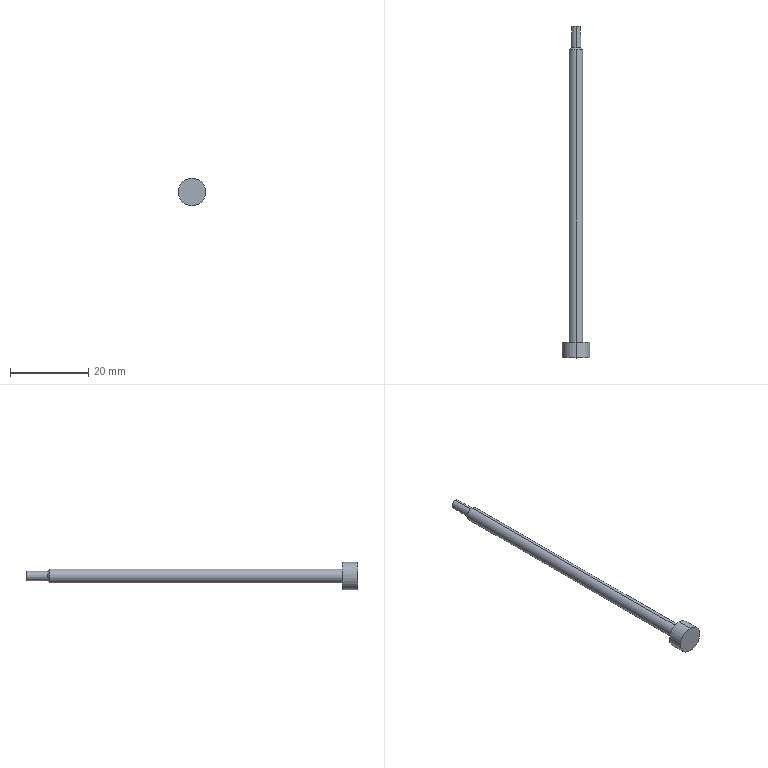Part | STEP file | 1 solid | 11 faces | box 7 x 84.723 x 7 mm | volume 901.172 mm3 | cylinder 4 | cone 4 | plane 3 | commonest cylinder face diameters 3.5 x2 7 x2
STEP:
#1=CARTESIAN_POINT('',(0.,0.,0.));
#2=DIRECTION('',(0.,0.,1.));
#3=DIRECTION('',(1.,0.,0.));
#4=AXIS2_PLACEMENT_3D('',#1,#2,#3);
#5=CARTESIAN_POINT('',(-48.742,-40.,118.07));
#6=VERTEX_POINT('',#5);
#7=CARTESIAN_POINT('',(-48.742,-40.,111.07));
#8=VERTEX_POINT('',#7);
#9=CARTESIAN_POINT('',(-48.742,-40.,114.57));
#10=DIRECTION('',(0.,1.,0.));
#11=DIRECTION('',(0.,0.,-1.));
#12=AXIS2_PLACEMENT_3D('',#9,#10,#11);
#13=CIRCLE('',#12,3.5);
#14=CARTESIAN_POINT('',(-48.742,-50.,114.57));
#15=DIRECTION('',(0.,1.,0.));
#16=DIRECTION('',(0.,0.,1.));
#17=AXIS2_PLACEMENT_3D('',#14,#15,#16);
#18=CYLINDRICAL_SURFACE('',#17,3.5);
#19=CARTESIAN_POINT('',(-3.142,10.));
#20=DIRECTION('',(1.,0.));
#21=VECTOR('',#20,1.);
#22=LINE('',#19,#21);
#23=(GEOMETRIC_REPRESENTATION_CONTEXT(2)PARAMETRIC_REPRESENTATION_CONTEXT()REPRESENTATION_CONTEXT('',''));
#24=DEFINITIONAL_REPRESENTATION('',(#22),#23);
#25=PCURVE('',#18,#24);
#26=CARTESIAN_POINT('',(-72.862,-40.,23.556));
#27=DIRECTION('',(0.,-1.,0.));
#28=DIRECTION('',(0.,0.,-1.));
#29=AXIS2_PLACEMENT_3D('',#26,#27,#28);
#30=PLANE('',#29);
#31=CARTESIAN_POINT('',(-87.514,24.12));
#32=CARTESIAN_POINT('',(-87.514,18.058));
#33=CARTESIAN_POINT('',(-92.764,21.089));
#34=CARTESIAN_POINT('',(-98.014,24.12));
#35=CARTESIAN_POINT('',(-92.764,27.151));
#36=CARTESIAN_POINT('',(-87.514,30.182));
#37=CARTESIAN_POINT('',(-87.514,24.12));
#38=(BOUNDED_CURVE()B_SPLINE_CURVE(2,(#31,#32,#33,#34,#35,#36,#37),.UNSPECIFIED.,.T.,.F.)B_SPLINE_CURVE_WITH_KNOTS((1,2,2,2,2,1),(-2.094,0.,2.094,4.189,6.283,8.378),.UNSPECIFIED.)CURVE()GEOMETRIC_REPRESENTATION_ITEM()RATIONAL_B_SPLINE_CURVE((1.,0.5,1.,0.5,1.,0.5,1.))REPRESENTATION_ITEM(''));
#39=(GEOMETRIC_REPRESENTATION_CONTEXT(2)PARAMETRIC_REPRESENTATION_CONTEXT()REPRESENTATION_CONTEXT('',''));
#40=DEFINITIONAL_REPRESENTATION('',(#38),#39);
#41=PCURVE('',#30,#40);
#42=SURFACE_CURVE('',#13,(#25,#41),.PCURVE_S1.);
#43=EDGE_CURVE('',#6,#8,#42,.T.);
#44=ORIENTED_EDGE('',*,*,#43,.T.);
#45=CARTESIAN_POINT('',(-48.742,-36.,111.07));
#46=VERTEX_POINT('',#45);
#47=CARTESIAN_POINT('',(-48.742,-50.,111.07));
#48=DIRECTION('',(0.,1.,0.));
#49=VECTOR('',#48,1.);
#50=LINE('',#47,#49);
#51=CARTESIAN_POINT('',(3.142,0.));
#52=DIRECTION('',(0.,1.));
#53=VECTOR('',#52,1.);
#54=LINE('',#51,#53);
#55=(GEOMETRIC_REPRESENTATION_CONTEXT(2)PARAMETRIC_REPRESENTATION_CONTEXT()REPRESENTATION_CONTEXT('',''));
#56=DEFINITIONAL_REPRESENTATION('',(#54),#55);
#57=PCURVE('',#18,#56);
#58=CARTESIAN_POINT('',(-48.742,-50.,114.57));
#59=DIRECTION('',(0.,1.,0.));
#60=DIRECTION('',(0.,0.,1.));
#61=AXIS2_PLACEMENT_3D('',#58,#59,#60);
#62=CYLINDRICAL_SURFACE('',#61,3.5);
#63=CARTESIAN_POINT('',(3.142,0.));
#64=DIRECTION('',(0.,1.));
#65=VECTOR('',#64,1.);
#66=LINE('',#63,#65);
#67=(GEOMETRIC_REPRESENTATION_CONTEXT(2)PARAMETRIC_REPRESENTATION_CONTEXT()REPRESENTATION_CONTEXT('',''));
#68=DEFINITIONAL_REPRESENTATION('',(#66),#67);
#69=PCURVE('',#62,#68);
#70=SURFACE_CURVE('',#50,(#57,#69),.PCURVE_S1.);
#71=EDGE_CURVE('',#8,#46,#70,.T.);
#72=ORIENTED_EDGE('',*,*,#71,.T.);
#73=CARTESIAN_POINT('',(-48.742,-36.,118.07));
#74=VERTEX_POINT('',#73);
#75=CARTESIAN_POINT('',(-48.742,-36.,114.57));
#76=DIRECTION('',(0.,-1.,0.));
#77=DIRECTION('',(0.,0.,-1.));
#78=AXIS2_PLACEMENT_3D('',#75,#76,#77);
#79=CIRCLE('',#78,3.5);
#80=CARTESIAN_POINT('',(3.142,14.));
#81=DIRECTION('',(-1.,0.));
#82=VECTOR('',#81,1.);
#83=LINE('',#80,#82);
#84=(GEOMETRIC_REPRESENTATION_CONTEXT(2)PARAMETRIC_REPRESENTATION_CONTEXT()REPRESENTATION_CONTEXT('',''));
#85=DEFINITIONAL_REPRESENTATION('',(#83),#84);
#86=PCURVE('',#18,#85);
#87=CARTESIAN_POINT('',(-48.742,-36.,114.57));
#88=DIRECTION('',(0.,1.,0.));
#89=DIRECTION('',(0.,0.,1.));
#90=AXIS2_PLACEMENT_3D('',#87,#88,#89);
#91=PLANE('',#90);
#92=CARTESIAN_POINT('',(-3.5,0.));
#93=CARTESIAN_POINT('',(-3.5,6.062));
#94=CARTESIAN_POINT('',(1.75,3.031));
#95=CARTESIAN_POINT('',(7.,0.));
#96=CARTESIAN_POINT('',(1.75,-3.031));
#97=CARTESIAN_POINT('',(-3.5,-6.062));
#98=CARTESIAN_POINT('',(-3.5,0.));
#99=(BOUNDED_CURVE()B_SPLINE_CURVE(2,(#92,#93,#94,#95,#96,#97,#98),.UNSPECIFIED.,.T.,.F.)B_SPLINE_CURVE_WITH_KNOTS((1,2,2,2,2,1),(-2.094,0.,2.094,4.189,6.283,8.378),.UNSPECIFIED.)CURVE()GEOMETRIC_REPRESENTATION_ITEM()RATIONAL_B_SPLINE_CURVE((1.,0.5,1.,0.5,1.,0.5,1.))REPRESENTATION_ITEM(''));
#100=(GEOMETRIC_REPRESENTATION_CONTEXT(2)PARAMETRIC_REPRESENTATION_CONTEXT()REPRESENTATION_CONTEXT('',''));
#101=DEFINITIONAL_REPRESENTATION('',(#99),#100);
#102=PCURVE('',#91,#101);
#103=SURFACE_CURVE('',#79,(#86,#102),.PCURVE_S1.);
#104=EDGE_CURVE('',#46,#74,#103,.T.);
#105=ORIENTED_EDGE('',*,*,#104,.T.);
#106=CARTESIAN_POINT('',(-48.742,-50.,118.07));
#107=DIRECTION('',(0.,1.,0.));
#108=VECTOR('',#107,1.);
#109=LINE('',#106,#108);
#110=CARTESIAN_POINT('',(0.,0.));
#111=DIRECTION('',(0.,1.));
#112=VECTOR('',#111,1.);
#113=LINE('',#110,#112);
#114=(GEOMETRIC_REPRESENTATION_CONTEXT(2)PARAMETRIC_REPRESENTATION_CONTEXT()REPRESENTATION_CONTEXT('',''));
#115=DEFINITIONAL_REPRESENTATION('',(#113),#114);
#116=PCURVE('',#18,#115);
#117=CARTESIAN_POINT('',(6.283,0.));
#118=DIRECTION('',(0.,1.));
#119=VECTOR('',#118,1.);
#120=LINE('',#117,#119);
#121=(GEOMETRIC_REPRESENTATION_CONTEXT(2)PARAMETRIC_REPRESENTATION_CONTEXT()REPRESENTATION_CONTEXT('',''));
#122=DEFINITIONAL_REPRESENTATION('',(#120),#121);
#123=PCURVE('',#62,#122);
#124=SURFACE_CURVE('',#109,(#116,#123),.PCURVE_S1.);
#125=EDGE_CURVE('',#6,#74,#124,.T.);
#126=ORIENTED_EDGE('',*,*,#125,.F.);
#127=EDGE_LOOP('',(#44,#72,#105,#126));
#128=FACE_BOUND('',#127,.T.);
#129=ADVANCED_FACE('',(#128),#18,.T.);
#130=CARTESIAN_POINT('',(-48.742,38.701,116.32));
#131=VERTEX_POINT('',#130);
#132=CARTESIAN_POINT('',(-48.742,38.701,112.82));
#133=VERTEX_POINT('',#132);
#134=CARTESIAN_POINT('',(-48.742,38.701,114.57));
#135=DIRECTION('',(0.,1.,0.));
#136=DIRECTION('',(0.,0.,-1.));
#137=AXIS2_PLACEMENT_3D('',#134,#135,#136);
#138=CIRCLE('',#137,1.75);
#139=CARTESIAN_POINT('',(-48.742,44.722,114.57));
#140=DIRECTION('',(0.,-1.,0.));
#141=DIRECTION('',(0.,0.,-1.));
#142=AXIS2_PLACEMENT_3D('',#139,#140,#141);
#143=CYLINDRICAL_SURFACE('',#142,1.75);
#144=CARTESIAN_POINT('',(6.283,6.021));
#145=DIRECTION('',(-1.,0.));
#146=VECTOR('',#145,1.);
#147=LINE('',#144,#146);
#148=(GEOMETRIC_REPRESENTATION_CONTEXT(2)PARAMETRIC_REPRESENTATION_CONTEXT()REPRESENTATION_CONTEXT('',''));
#149=DEFINITIONAL_REPRESENTATION('',(#147),#148);
#150=PCURVE('',#143,#149);
#151=CARTESIAN_POINT('',(-48.742,39.204,114.57));
#152=DIRECTION('',(0.,-1.,0.));
#153=DIRECTION('',(0.,0.,-1.));
#154=AXIS2_PLACEMENT_3D('',#151,#152,#153);
#155=CONICAL_SURFACE('',#154,1.247,0.7854);
#156=CARTESIAN_POINT('',(6.283,0.5027));
#157=DIRECTION('',(-1.,0.));
#158=VECTOR('',#157,1.);
#159=LINE('',#156,#158);
#160=(GEOMETRIC_REPRESENTATION_CONTEXT(2)PARAMETRIC_REPRESENTATION_CONTEXT()REPRESENTATION_CONTEXT('',''));
#161=DEFINITIONAL_REPRESENTATION('',(#159),#160);
#162=PCURVE('',#155,#161);
#163=SURFACE_CURVE('',#138,(#150,#162),.PCURVE_S1.);
#164=EDGE_CURVE('',#131,#133,#163,.T.);
#165=ORIENTED_EDGE('',*,*,#164,.F.);
#166=CARTESIAN_POINT('',(-48.742,-36.,116.32));
#167=VERTEX_POINT('',#166);
#168=CARTESIAN_POINT('',(-48.742,44.722,116.32));
#169=DIRECTION('',(0.,-1.,0.));
#170=VECTOR('',#169,1.);
#171=LINE('',#168,#170);
#172=CARTESIAN_POINT('',(3.142,0.));
#173=DIRECTION('',(0.,1.));
#174=VECTOR('',#173,1.);
#175=LINE('',#172,#174);
#176=(GEOMETRIC_REPRESENTATION_CONTEXT(2)PARAMETRIC_REPRESENTATION_CONTEXT()REPRESENTATION_CONTEXT('',''));
#177=DEFINITIONAL_REPRESENTATION('',(#175),#176);
#178=PCURVE('',#143,#177);
#179=CARTESIAN_POINT('',(-48.742,44.722,114.57));
#180=DIRECTION('',(0.,-1.,0.));
#181=DIRECTION('',(0.,0.,-1.));
#182=AXIS2_PLACEMENT_3D('',#179,#180,#181);
#183=CYLINDRICAL_SURFACE('',#182,1.75);
#184=CARTESIAN_POINT('',(3.142,0.));
#185=DIRECTION('',(0.,1.));
#186=VECTOR('',#185,1.);
#187=LINE('',#184,#186);
#188=(GEOMETRIC_REPRESENTATION_CONTEXT(2)PARAMETRIC_REPRESENTATION_CONTEXT()REPRESENTATION_CONTEXT('',''));
#189=DEFINITIONAL_REPRESENTATION('',(#187),#188);
#190=PCURVE('',#183,#189);
#191=SURFACE_CURVE('',#171,(#178,#190),.PCURVE_S1.);
#192=EDGE_CURVE('',#131,#167,#191,.T.);
#193=ORIENTED_EDGE('',*,*,#192,.T.);
#194=CARTESIAN_POINT('',(-48.742,-36.,112.82));
#195=VERTEX_POINT('',#194);
#196=CARTESIAN_POINT('',(-48.742,-36.,114.57));
#197=DIRECTION('',(0.,-1.,0.));
#198=DIRECTION('',(0.,0.,1.));
#199=AXIS2_PLACEMENT_3D('',#196,#197,#198);
#200=CIRCLE('',#199,1.75);
#201=CARTESIAN_POINT('',(-3.142,80.722));
#202=DIRECTION('',(1.,0.));
#203=VECTOR('',#202,1.);
#204=LINE('',#201,#203);
#205=(GEOMETRIC_REPRESENTATION_CONTEXT(2)PARAMETRIC_REPRESENTATION_CONTEXT()REPRESENTATION_CONTEXT('',''));
#206=DEFINITIONAL_REPRESENTATION('',(#204),#205);
#207=PCURVE('',#143,#206);
#208=CARTESIAN_POINT('',(1.75,0.));
#209=CARTESIAN_POINT('',(1.75,-3.031));
#210=CARTESIAN_POINT('',(-0.875,-1.516));
#211=CARTESIAN_POINT('',(-3.5,0.));
#212=CARTESIAN_POINT('',(-0.875,1.516));
#213=CARTESIAN_POINT('',(1.75,3.031));
#214=CARTESIAN_POINT('',(1.75,0.));
#215=(BOUNDED_CURVE()B_SPLINE_CURVE(2,(#208,#209,#210,#211,#212,#213,#214),.UNSPECIFIED.,.T.,.F.)B_SPLINE_CURVE_WITH_KNOTS((1,2,2,2,2,1),(-2.094,0.,2.094,4.189,6.283,8.378),.UNSPECIFIED.)CURVE()GEOMETRIC_REPRESENTATION_ITEM()RATIONAL_B_SPLINE_CURVE((1.,0.5,1.,0.5,1.,0.5,1.))REPRESENTATION_ITEM(''));
#216=(GEOMETRIC_REPRESENTATION_CONTEXT(2)PARAMETRIC_REPRESENTATION_CONTEXT()REPRESENTATION_CONTEXT('',''));
#217=DEFINITIONAL_REPRESENTATION('',(#215),#216);
#218=PCURVE('',#91,#217);
#219=SURFACE_CURVE('',#200,(#207,#218),.PCURVE_S1.);
#220=EDGE_CURVE('',#195,#167,#219,.T.);
#221=ORIENTED_EDGE('',*,*,#220,.F.);
#222=CARTESIAN_POINT('',(-48.742,44.722,112.82));
#223=DIRECTION('',(0.,-1.,0.));
#224=VECTOR('',#223,1.);
#225=LINE('',#222,#224);
#226=CARTESIAN_POINT('',(0.,0.));
#227=DIRECTION('',(0.,1.));
#228=VECTOR('',#227,1.);
#229=LINE('',#226,#228);
#230=(GEOMETRIC_REPRESENTATION_CONTEXT(2)PARAMETRIC_REPRESENTATION_CONTEXT()REPRESENTATION_CONTEXT('',''));
#231=DEFINITIONAL_REPRESENTATION('',(#229),#230);
#232=PCURVE('',#143,#231);
#233=CARTESIAN_POINT('',(6.283,0.));
#234=DIRECTION('',(0.,1.));
#235=VECTOR('',#234,1.);
#236=LINE('',#233,#235);
#237=(GEOMETRIC_REPRESENTATION_CONTEXT(2)PARAMETRIC_REPRESENTATION_CONTEXT()REPRESENTATION_CONTEXT('',''));
#238=DEFINITIONAL_REPRESENTATION('',(#236),#237);
#239=PCURVE('',#183,#238);
#240=SURFACE_CURVE('',#225,(#232,#239),.PCURVE_S1.);
#241=EDGE_CURVE('',#133,#195,#240,.T.);
#242=ORIENTED_EDGE('',*,*,#241,.F.);
#243=EDGE_LOOP('',(#165,#193,#221,#242));
#244=FACE_BOUND('',#243,.T.);
#245=ADVANCED_FACE('',(#244),#143,.T.);
#246=CARTESIAN_POINT('',(-48.742,39.204,113.323));
#247=VERTEX_POINT('',#246);
#248=CARTESIAN_POINT('',(-48.742,39.204,115.817));
#249=VERTEX_POINT('',#248);
#250=CARTESIAN_POINT('',(-48.742,39.204,114.57));
#251=DIRECTION('',(0.,-1.,0.));
#252=DIRECTION('',(0.,0.,-1.));
#253=AXIS2_PLACEMENT_3D('',#250,#251,#252);
#254=CIRCLE('',#253,1.247);
#255=CARTESIAN_POINT('',(0.,0.));
#256=DIRECTION('',(1.,0.));
#257=VECTOR('',#256,1.);
#258=LINE('',#255,#257);
#259=(GEOMETRIC_REPRESENTATION_CONTEXT(2)PARAMETRIC_REPRESENTATION_CONTEXT()REPRESENTATION_CONTEXT('',''));
#260=DEFINITIONAL_REPRESENTATION('',(#258),#259);
#261=PCURVE('',#155,#260);
#262=CARTESIAN_POINT('',(-48.742,38.693,114.57));
#263=DIRECTION('',(0.,-1.,0.));
#264=DIRECTION('',(0.,0.,-1.));
#265=AXIS2_PLACEMENT_3D('',#262,#263,#264);
#266=CONICAL_SURFACE('',#265,1.256,0.01745);
#267=CARTESIAN_POINT('',(0.,-0.5114));
#268=DIRECTION('',(1.,0.));
#269=VECTOR('',#268,1.);
#270=LINE('',#267,#269);
#271=(GEOMETRIC_REPRESENTATION_CONTEXT(2)PARAMETRIC_REPRESENTATION_CONTEXT()REPRESENTATION_CONTEXT('',''));
#272=DEFINITIONAL_REPRESENTATION('',(#270),#271);
#273=PCURVE('',#266,#272);
#274=SURFACE_CURVE('',#254,(#261,#273),.PCURVE_S1.);
#275=EDGE_CURVE('',#247,#249,#274,.T.);
#276=ORIENTED_EDGE('',*,*,#275,.T.);
#277=CARTESIAN_POINT('',(-48.742,39.204,115.817));
#278=DIRECTION('',(0.,-0.7071,0.7071));
#279=VECTOR('',#278,1.);
#280=LINE('',#277,#279);
#281=CARTESIAN_POINT('',(3.142,0.));
#282=DIRECTION('',(0.,1.));
#283=VECTOR('',#282,1.);
#284=LINE('',#281,#283);
#285=(GEOMETRIC_REPRESENTATION_CONTEXT(2)PARAMETRIC_REPRESENTATION_CONTEXT()REPRESENTATION_CONTEXT('',''));
#286=DEFINITIONAL_REPRESENTATION('',(#284),#285);
#287=PCURVE('',#155,#286);
#288=CARTESIAN_POINT('',(-48.742,39.204,114.57));
#289=DIRECTION('',(0.,-1.,0.));
#290=DIRECTION('',(0.,0.,-1.));
#291=AXIS2_PLACEMENT_3D('',#288,#289,#290);
#292=CONICAL_SURFACE('',#291,1.247,0.7854);
#293=CARTESIAN_POINT('',(3.142,0.));
#294=DIRECTION('',(0.,1.));
#295=VECTOR('',#294,1.);
#296=LINE('',#293,#295);
#297=(GEOMETRIC_REPRESENTATION_CONTEXT(2)PARAMETRIC_REPRESENTATION_CONTEXT()REPRESENTATION_CONTEXT('',''));
#298=DEFINITIONAL_REPRESENTATION('',(#296),#297);
#299=PCURVE('',#292,#298);
#300=SURFACE_CURVE('',#280,(#287,#299),.PCURVE_S1.);
#301=EDGE_CURVE('',#249,#131,#300,.T.);
#302=ORIENTED_EDGE('',*,*,#301,.T.);
#303=ORIENTED_EDGE('',*,*,#164,.T.);
#304=CARTESIAN_POINT('',(-48.742,39.204,113.323));
#305=DIRECTION('',(0.,-0.7071,-0.7071));
#306=VECTOR('',#305,1.);
#307=LINE('',#304,#306);
#308=CARTESIAN_POINT('',(0.,0.));
#309=DIRECTION('',(0.,1.));
#310=VECTOR('',#309,1.);
#311=LINE('',#308,#310);
#312=(GEOMETRIC_REPRESENTATION_CONTEXT(2)PARAMETRIC_REPRESENTATION_CONTEXT()REPRESENTATION_CONTEXT('',''));
#313=DEFINITIONAL_REPRESENTATION('',(#311),#312);
#314=PCURVE('',#155,#313);
#315=CARTESIAN_POINT('',(6.283,0.));
#316=DIRECTION('',(0.,1.));
#317=VECTOR('',#316,1.);
#318=LINE('',#315,#317);
#319=(GEOMETRIC_REPRESENTATION_CONTEXT(2)PARAMETRIC_REPRESENTATION_CONTEXT()REPRESENTATION_CONTEXT('',''));
#320=DEFINITIONAL_REPRESENTATION('',(#318),#319);
#321=PCURVE('',#292,#320);
#322=SURFACE_CURVE('',#307,(#314,#321),.PCURVE_S1.);
#323=EDGE_CURVE('',#247,#133,#322,.T.);
#324=ORIENTED_EDGE('',*,*,#323,.F.);
#325=EDGE_LOOP('',(#276,#302,#303,#324));
#326=FACE_BOUND('',#325,.T.);
#327=ADVANCED_FACE('',(#326),#155,.T.);
#328=CARTESIAN_POINT('',(-48.742,44.722,113.419));
#329=VERTEX_POINT('',#328);
#330=CARTESIAN_POINT('',(-48.742,44.722,115.721));
#331=VERTEX_POINT('',#330);
#332=CARTESIAN_POINT('',(-48.742,44.722,114.57));
#333=DIRECTION('',(0.,-1.,0.));
#334=DIRECTION('',(0.,0.,-1.));
#335=AXIS2_PLACEMENT_3D('',#332,#333,#334);
#336=CIRCLE('',#335,1.151);
#337=CARTESIAN_POINT('',(0.,-6.03));
#338=DIRECTION('',(1.,0.));
#339=VECTOR('',#338,1.);
#340=LINE('',#337,#339);
#341=(GEOMETRIC_REPRESENTATION_CONTEXT(2)PARAMETRIC_REPRESENTATION_CONTEXT()REPRESENTATION_CONTEXT('',''));
#342=DEFINITIONAL_REPRESENTATION('',(#340),#341);
#343=PCURVE('',#266,#342);
#344=CARTESIAN_POINT('',(-48.742,44.722,114.57));
#345=DIRECTION('',(0.,1.,0.));
#346=DIRECTION('',(0.,0.,1.));
#347=AXIS2_PLACEMENT_3D('',#344,#345,#346);
#348=PLANE('',#347);
#349=CARTESIAN_POINT('',(-1.151,0.));
#350=CARTESIAN_POINT('',(-1.151,1.994));
#351=CARTESIAN_POINT('',(0.5755,0.9968));
#352=CARTESIAN_POINT('',(2.302,0.));
#353=CARTESIAN_POINT('',(0.5755,-0.9968));
#354=CARTESIAN_POINT('',(-1.151,-1.994));
#355=CARTESIAN_POINT('',(-1.151,0.));
#356=(BOUNDED_CURVE()B_SPLINE_CURVE(2,(#349,#350,#351,#352,#353,#354,#355),.UNSPECIFIED.,.T.,.F.)B_SPLINE_CURVE_WITH_KNOTS((1,2,2,2,2,1),(-2.094,0.,2.094,4.189,6.283,8.378),.UNSPECIFIED.)CURVE()GEOMETRIC_REPRESENTATION_ITEM()RATIONAL_B_SPLINE_CURVE((1.,0.5,1.,0.5,1.,0.5,1.))REPRESENTATION_ITEM(''));
#357=(GEOMETRIC_REPRESENTATION_CONTEXT(2)PARAMETRIC_REPRESENTATION_CONTEXT()REPRESENTATION_CONTEXT('',''));
#358=DEFINITIONAL_REPRESENTATION('',(#356),#357);
#359=PCURVE('',#348,#358);
#360=SURFACE_CURVE('',#336,(#343,#359),.PCURVE_S1.);
#361=EDGE_CURVE('',#329,#331,#360,.T.);
#362=ORIENTED_EDGE('',*,*,#361,.T.);
#363=CARTESIAN_POINT('',(-48.742,38.693,115.826));
#364=DIRECTION('',(0.,-0.9998,0.01745));
#365=VECTOR('',#364,1.);
#366=LINE('',#363,#365);
#367=CARTESIAN_POINT('',(3.142,0.));
#368=DIRECTION('',(0.,1.));
#369=VECTOR('',#368,1.);
#370=LINE('',#367,#369);
#371=(GEOMETRIC_REPRESENTATION_CONTEXT(2)PARAMETRIC_REPRESENTATION_CONTEXT()REPRESENTATION_CONTEXT('',''));
#372=DEFINITIONAL_REPRESENTATION('',(#370),#371);
#373=PCURVE('',#266,#372);
#374=CARTESIAN_POINT('',(-48.742,38.693,114.57));
#375=DIRECTION('',(0.,-1.,0.));
#376=DIRECTION('',(0.,0.,-1.));
#377=AXIS2_PLACEMENT_3D('',#374,#375,#376);
#378=CONICAL_SURFACE('',#377,1.256,0.01745);
#379=CARTESIAN_POINT('',(3.142,0.));
#380=DIRECTION('',(0.,1.));
#381=VECTOR('',#380,1.);
#382=LINE('',#379,#381);
#383=(GEOMETRIC_REPRESENTATION_CONTEXT(2)PARAMETRIC_REPRESENTATION_CONTEXT()REPRESENTATION_CONTEXT('',''));
#384=DEFINITIONAL_REPRESENTATION('',(#382),#383);
#385=PCURVE('',#378,#384);
#386=SURFACE_CURVE('',#366,(#373,#385),.PCURVE_S1.);
#387=EDGE_CURVE('',#331,#249,#386,.T.);
#388=ORIENTED_EDGE('',*,*,#387,.T.);
#389=ORIENTED_EDGE('',*,*,#275,.F.);
#390=CARTESIAN_POINT('',(-48.742,38.693,113.314));
#391=DIRECTION('',(0.,-0.9998,-0.01745));
#392=VECTOR('',#391,1.);
#393=LINE('',#390,#392);
#394=CARTESIAN_POINT('',(0.,0.));
#395=DIRECTION('',(0.,1.));
#396=VECTOR('',#395,1.);
#397=LINE('',#394,#396);
#398=(GEOMETRIC_REPRESENTATION_CONTEXT(2)PARAMETRIC_REPRESENTATION_CONTEXT()REPRESENTATION_CONTEXT('',''));
#399=DEFINITIONAL_REPRESENTATION('',(#397),#398);
#400=PCURVE('',#266,#399);
#401=CARTESIAN_POINT('',(6.283,0.));
#402=DIRECTION('',(0.,1.));
#403=VECTOR('',#402,1.);
#404=LINE('',#401,#403);
#405=(GEOMETRIC_REPRESENTATION_CONTEXT(2)PARAMETRIC_REPRESENTATION_CONTEXT()REPRESENTATION_CONTEXT('',''));
#406=DEFINITIONAL_REPRESENTATION('',(#404),#405);
#407=PCURVE('',#378,#406);
#408=SURFACE_CURVE('',#393,(#400,#407),.PCURVE_S1.);
#409=EDGE_CURVE('',#329,#247,#408,.T.);
#410=ORIENTED_EDGE('',*,*,#409,.F.);
#411=EDGE_LOOP('',(#362,#388,#389,#410));
#412=FACE_BOUND('',#411,.T.);
#413=ADVANCED_FACE('',(#412),#266,.T.);
#414=ORIENTED_EDGE('',*,*,#387,.F.);
#415=CARTESIAN_POINT('',(-48.742,44.722,114.57));
#416=DIRECTION('',(0.,-1.,0.));
#417=DIRECTION('',(0.,0.,-1.));
#418=AXIS2_PLACEMENT_3D('',#415,#416,#417);
#419=CIRCLE('',#418,1.151);
#420=CARTESIAN_POINT('',(0.,-6.03));
#421=DIRECTION('',(1.,0.));
#422=VECTOR('',#421,1.);
#423=LINE('',#420,#422);
#424=(GEOMETRIC_REPRESENTATION_CONTEXT(2)PARAMETRIC_REPRESENTATION_CONTEXT()REPRESENTATION_CONTEXT('',''));
#425=DEFINITIONAL_REPRESENTATION('',(#423),#424);
#426=PCURVE('',#378,#425);
#427=CARTESIAN_POINT('',(-1.151,0.));
#428=CARTESIAN_POINT('',(-1.151,1.994));
#429=CARTESIAN_POINT('',(0.5755,0.9968));
#430=CARTESIAN_POINT('',(2.302,0.));
#431=CARTESIAN_POINT('',(0.5755,-0.9968));
#432=CARTESIAN_POINT('',(-1.151,-1.994));
#433=CARTESIAN_POINT('',(-1.151,0.));
#434=(BOUNDED_CURVE()B_SPLINE_CURVE(2,(#427,#428,#429,#430,#431,#432,#433),.UNSPECIFIED.,.T.,.F.)B_SPLINE_CURVE_WITH_KNOTS((1,2,2,2,2,1),(-2.094,0.,2.094,4.189,6.283,8.378),.UNSPECIFIED.)CURVE()GEOMETRIC_REPRESENTATION_ITEM()RATIONAL_B_SPLINE_CURVE((1.,0.5,1.,0.5,1.,0.5,1.))REPRESENTATION_ITEM(''));
#435=(GEOMETRIC_REPRESENTATION_CONTEXT(2)PARAMETRIC_REPRESENTATION_CONTEXT()REPRESENTATION_CONTEXT('',''));
#436=DEFINITIONAL_REPRESENTATION('',(#434),#435);
#437=PCURVE('',#348,#436);
#438=SURFACE_CURVE('',#419,(#426,#437),.PCURVE_S1.);
#439=EDGE_CURVE('',#331,#329,#438,.T.);
#440=ORIENTED_EDGE('',*,*,#439,.T.);
#441=ORIENTED_EDGE('',*,*,#409,.T.);
#442=CARTESIAN_POINT('',(-48.742,39.204,114.57));
#443=DIRECTION('',(0.,-1.,0.));
#444=DIRECTION('',(0.,0.,-1.));
#445=AXIS2_PLACEMENT_3D('',#442,#443,#444);
#446=CIRCLE('',#445,1.247);
#447=CARTESIAN_POINT('',(0.,-0.5114));
#448=DIRECTION('',(1.,0.));
#449=VECTOR('',#448,1.);
#450=LINE('',#447,#449);
#451=(GEOMETRIC_REPRESENTATION_CONTEXT(2)PARAMETRIC_REPRESENTATION_CONTEXT()REPRESENTATION_CONTEXT('',''));
#452=DEFINITIONAL_REPRESENTATION('',(#450),#451);
#453=PCURVE('',#378,#452);
#454=CARTESIAN_POINT('',(0.,0.));
#455=DIRECTION('',(1.,0.));
#456=VECTOR('',#455,1.);
#457=LINE('',#454,#456);
#458=(GEOMETRIC_REPRESENTATION_CONTEXT(2)PARAMETRIC_REPRESENTATION_CONTEXT()REPRESENTATION_CONTEXT('',''));
#459=DEFINITIONAL_REPRESENTATION('',(#457),#458);
#460=PCURVE('',#292,#459);
#461=SURFACE_CURVE('',#446,(#453,#460),.PCURVE_S1.);
#462=EDGE_CURVE('',#249,#247,#461,.T.);
#463=ORIENTED_EDGE('',*,*,#462,.F.);
#464=EDGE_LOOP('',(#414,#440,#441,#463));
#465=FACE_BOUND('',#464,.T.);
#466=ADVANCED_FACE('',(#465),#378,.T.);
#467=ORIENTED_EDGE('',*,*,#301,.F.);
#468=ORIENTED_EDGE('',*,*,#462,.T.);
#469=ORIENTED_EDGE('',*,*,#323,.T.);
#470=CARTESIAN_POINT('',(-48.742,38.701,114.57));
#471=DIRECTION('',(0.,1.,0.));
#472=DIRECTION('',(0.,0.,-1.));
#473=AXIS2_PLACEMENT_3D('',#470,#471,#472);
#474=CIRCLE('',#473,1.75);
#475=CARTESIAN_POINT('',(6.283,0.5027));
#476=DIRECTION('',(-1.,0.));
#477=VECTOR('',#476,1.);
#478=LINE('',#475,#477);
#479=(GEOMETRIC_REPRESENTATION_CONTEXT(2)PARAMETRIC_REPRESENTATION_CONTEXT()REPRESENTATION_CONTEXT('',''));
#480=DEFINITIONAL_REPRESENTATION('',(#478),#479);
#481=PCURVE('',#292,#480);
#482=CARTESIAN_POINT('',(6.283,6.021));
#483=DIRECTION('',(-1.,0.));
#484=VECTOR('',#483,1.);
#485=LINE('',#482,#484);
#486=(GEOMETRIC_REPRESENTATION_CONTEXT(2)PARAMETRIC_REPRESENTATION_CONTEXT()REPRESENTATION_CONTEXT('',''));
#487=DEFINITIONAL_REPRESENTATION('',(#485),#486);
#488=PCURVE('',#183,#487);
#489=SURFACE_CURVE('',#474,(#481,#488),.PCURVE_S1.);
#490=EDGE_CURVE('',#133,#131,#489,.T.);
#491=ORIENTED_EDGE('',*,*,#490,.T.);
#492=EDGE_LOOP('',(#467,#468,#469,#491));
#493=FACE_BOUND('',#492,.T.);
#494=ADVANCED_FACE('',(#493),#292,.T.);
#495=ORIENTED_EDGE('',*,*,#192,.F.);
#496=ORIENTED_EDGE('',*,*,#490,.F.);
#497=ORIENTED_EDGE('',*,*,#241,.T.);
#498=CARTESIAN_POINT('',(-48.742,-36.,114.57));
#499=DIRECTION('',(0.,-1.,0.));
#500=DIRECTION('',(0.,0.,1.));
#501=AXIS2_PLACEMENT_3D('',#498,#499,#500);
#502=CIRCLE('',#501,1.75);
#503=CARTESIAN_POINT('',(3.142,80.722));
#504=DIRECTION('',(1.,0.));
#505=VECTOR('',#504,1.);
#506=LINE('',#503,#505);
#507=(GEOMETRIC_REPRESENTATION_CONTEXT(2)PARAMETRIC_REPRESENTATION_CONTEXT()REPRESENTATION_CONTEXT('',''));
#508=DEFINITIONAL_REPRESENTATION('',(#506),#507);
#509=PCURVE('',#183,#508);
#510=CARTESIAN_POINT('',(1.75,0.));
#511=CARTESIAN_POINT('',(1.75,-3.031));
#512=CARTESIAN_POINT('',(-0.875,-1.516));
#513=CARTESIAN_POINT('',(-3.5,0.));
#514=CARTESIAN_POINT('',(-0.875,1.516));
#515=CARTESIAN_POINT('',(1.75,3.031));
#516=CARTESIAN_POINT('',(1.75,0.));
#517=(BOUNDED_CURVE()B_SPLINE_CURVE(2,(#510,#511,#512,#513,#514,#515,#516),.UNSPECIFIED.,.T.,.F.)B_SPLINE_CURVE_WITH_KNOTS((1,2,2,2,2,1),(-2.094,0.,2.094,4.189,6.283,8.378),.UNSPECIFIED.)CURVE()GEOMETRIC_REPRESENTATION_ITEM()RATIONAL_B_SPLINE_CURVE((1.,0.5,1.,0.5,1.,0.5,1.))REPRESENTATION_ITEM(''));
#518=(GEOMETRIC_REPRESENTATION_CONTEXT(2)PARAMETRIC_REPRESENTATION_CONTEXT()REPRESENTATION_CONTEXT('',''));
#519=DEFINITIONAL_REPRESENTATION('',(#517),#518);
#520=PCURVE('',#91,#519);
#521=SURFACE_CURVE('',#502,(#509,#520),.PCURVE_S1.);
#522=EDGE_CURVE('',#167,#195,#521,.T.);
#523=ORIENTED_EDGE('',*,*,#522,.F.);
#524=EDGE_LOOP('',(#495,#496,#497,#523));
#525=FACE_BOUND('',#524,.T.);
#526=ADVANCED_FACE('',(#525),#183,.T.);
#527=ORIENTED_EDGE('',*,*,#361,.F.);
#528=ORIENTED_EDGE('',*,*,#439,.F.);
#529=EDGE_LOOP('',(#527,#528));
#530=FACE_BOUND('',#529,.T.);
#531=ADVANCED_FACE('',(#530),#348,.T.);
#532=ORIENTED_EDGE('',*,*,#220,.T.);
#533=ORIENTED_EDGE('',*,*,#522,.T.);
#534=EDGE_LOOP('',(#532,#533));
#535=FACE_BOUND('',#534,.T.);
#536=CARTESIAN_POINT('',(-48.742,-36.,114.57));
#537=DIRECTION('',(0.,-1.,0.));
#538=DIRECTION('',(0.,0.,-1.));
#539=AXIS2_PLACEMENT_3D('',#536,#537,#538);
#540=CIRCLE('',#539,3.5);
#541=CARTESIAN_POINT('',(-3.5,0.));
#542=CARTESIAN_POINT('',(-3.5,6.062));
#543=CARTESIAN_POINT('',(1.75,3.031));
#544=CARTESIAN_POINT('',(7.,0.));
#545=CARTESIAN_POINT('',(1.75,-3.031));
#546=CARTESIAN_POINT('',(-3.5,-6.062));
#547=CARTESIAN_POINT('',(-3.5,0.));
#548=(BOUNDED_CURVE()B_SPLINE_CURVE(2,(#541,#542,#543,#544,#545,#546,#547),.UNSPECIFIED.,.T.,.F.)B_SPLINE_CURVE_WITH_KNOTS((1,2,2,2,2,1),(-2.094,0.,2.094,4.189,6.283,8.378),.UNSPECIFIED.)CURVE()GEOMETRIC_REPRESENTATION_ITEM()RATIONAL_B_SPLINE_CURVE((1.,0.5,1.,0.5,1.,0.5,1.))REPRESENTATION_ITEM(''));
#549=(GEOMETRIC_REPRESENTATION_CONTEXT(2)PARAMETRIC_REPRESENTATION_CONTEXT()REPRESENTATION_CONTEXT('',''));
#550=DEFINITIONAL_REPRESENTATION('',(#548),#549);
#551=PCURVE('',#91,#550);
#552=CARTESIAN_POINT('',(9.425,14.));
#553=DIRECTION('',(-1.,0.));
#554=VECTOR('',#553,1.);
#555=LINE('',#552,#554);
#556=(GEOMETRIC_REPRESENTATION_CONTEXT(2)PARAMETRIC_REPRESENTATION_CONTEXT()REPRESENTATION_CONTEXT('',''));
#557=DEFINITIONAL_REPRESENTATION('',(#555),#556);
#558=PCURVE('',#62,#557);
#559=SURFACE_CURVE('',#540,(#551,#558),.PCURVE_S1.);
#560=EDGE_CURVE('',#74,#46,#559,.T.);
#561=ORIENTED_EDGE('',*,*,#560,.F.);
#562=ORIENTED_EDGE('',*,*,#104,.F.);
#563=EDGE_LOOP('',(#561,#562));
#564=FACE_BOUND('',#563,.T.);
#565=ADVANCED_FACE('',(#535,#564),#91,.T.);
#566=ORIENTED_EDGE('',*,*,#71,.F.);
#567=CARTESIAN_POINT('',(-48.742,-40.,114.57));
#568=DIRECTION('',(0.,1.,0.));
#569=DIRECTION('',(0.,0.,-1.));
#570=AXIS2_PLACEMENT_3D('',#567,#568,#569);
#571=CIRCLE('',#570,3.5);
#572=CARTESIAN_POINT('',(3.142,10.));
#573=DIRECTION('',(1.,0.));
#574=VECTOR('',#573,1.);
#575=LINE('',#572,#574);
#576=(GEOMETRIC_REPRESENTATION_CONTEXT(2)PARAMETRIC_REPRESENTATION_CONTEXT()REPRESENTATION_CONTEXT('',''));
#577=DEFINITIONAL_REPRESENTATION('',(#575),#576);
#578=PCURVE('',#62,#577);
#579=CARTESIAN_POINT('',(-87.514,24.12));
#580=CARTESIAN_POINT('',(-87.514,18.058));
#581=CARTESIAN_POINT('',(-92.764,21.089));
#582=CARTESIAN_POINT('',(-98.014,24.12));
#583=CARTESIAN_POINT('',(-92.764,27.151));
#584=CARTESIAN_POINT('',(-87.514,30.182));
#585=CARTESIAN_POINT('',(-87.514,24.12));
#586=(BOUNDED_CURVE()B_SPLINE_CURVE(2,(#579,#580,#581,#582,#583,#584,#585),.UNSPECIFIED.,.T.,.F.)B_SPLINE_CURVE_WITH_KNOTS((1,2,2,2,2,1),(-2.094,0.,2.094,4.189,6.283,8.378),.UNSPECIFIED.)CURVE()GEOMETRIC_REPRESENTATION_ITEM()RATIONAL_B_SPLINE_CURVE((1.,0.5,1.,0.5,1.,0.5,1.))REPRESENTATION_ITEM(''));
#587=(GEOMETRIC_REPRESENTATION_CONTEXT(2)PARAMETRIC_REPRESENTATION_CONTEXT()REPRESENTATION_CONTEXT('',''));
#588=DEFINITIONAL_REPRESENTATION('',(#586),#587);
#589=PCURVE('',#30,#588);
#590=SURFACE_CURVE('',#571,(#578,#589),.PCURVE_S1.);
#591=EDGE_CURVE('',#8,#6,#590,.T.);
#592=ORIENTED_EDGE('',*,*,#591,.T.);
#593=ORIENTED_EDGE('',*,*,#125,.T.);
#594=ORIENTED_EDGE('',*,*,#560,.T.);
#595=EDGE_LOOP('',(#566,#592,#593,#594));
#596=FACE_BOUND('',#595,.T.);
#597=ADVANCED_FACE('',(#596),#62,.T.);
#598=ORIENTED_EDGE('',*,*,#43,.F.);
#599=ORIENTED_EDGE('',*,*,#591,.F.);
#600=EDGE_LOOP('',(#598,#599));
#601=FACE_BOUND('',#600,.T.);
#602=ADVANCED_FACE('',(#601),#30,.T.);
#603=CLOSED_SHELL('',(#129,#245,#327,#413,#466,#494,#526,#531,#565,#597,#602));
#604=MANIFOLD_SOLID_BREP('',#603);
#605=(LENGTH_UNIT()NAMED_UNIT(*)SI_UNIT(.MILLI.,.METRE.));
#606=UNCERTAINTY_MEASURE_WITH_UNIT(LENGTH_MEASURE(0.0000001),#605,'','');
#607=(NAMED_UNIT(*)PLANE_ANGLE_UNIT()SI_UNIT($,.RADIAN.));
#608=(NAMED_UNIT(*)SI_UNIT($,.STERADIAN.)SOLID_ANGLE_UNIT());
#609=(GEOMETRIC_REPRESENTATION_CONTEXT(3)GLOBAL_UNCERTAINTY_ASSIGNED_CONTEXT((#606))GLOBAL_UNIT_ASSIGNED_CONTEXT((#605,#607,#608))REPRESENTATION_CONTEXT('',''));
#610=ADVANCED_BREP_SHAPE_REPRESENTATION('',(#4,#604),#609);